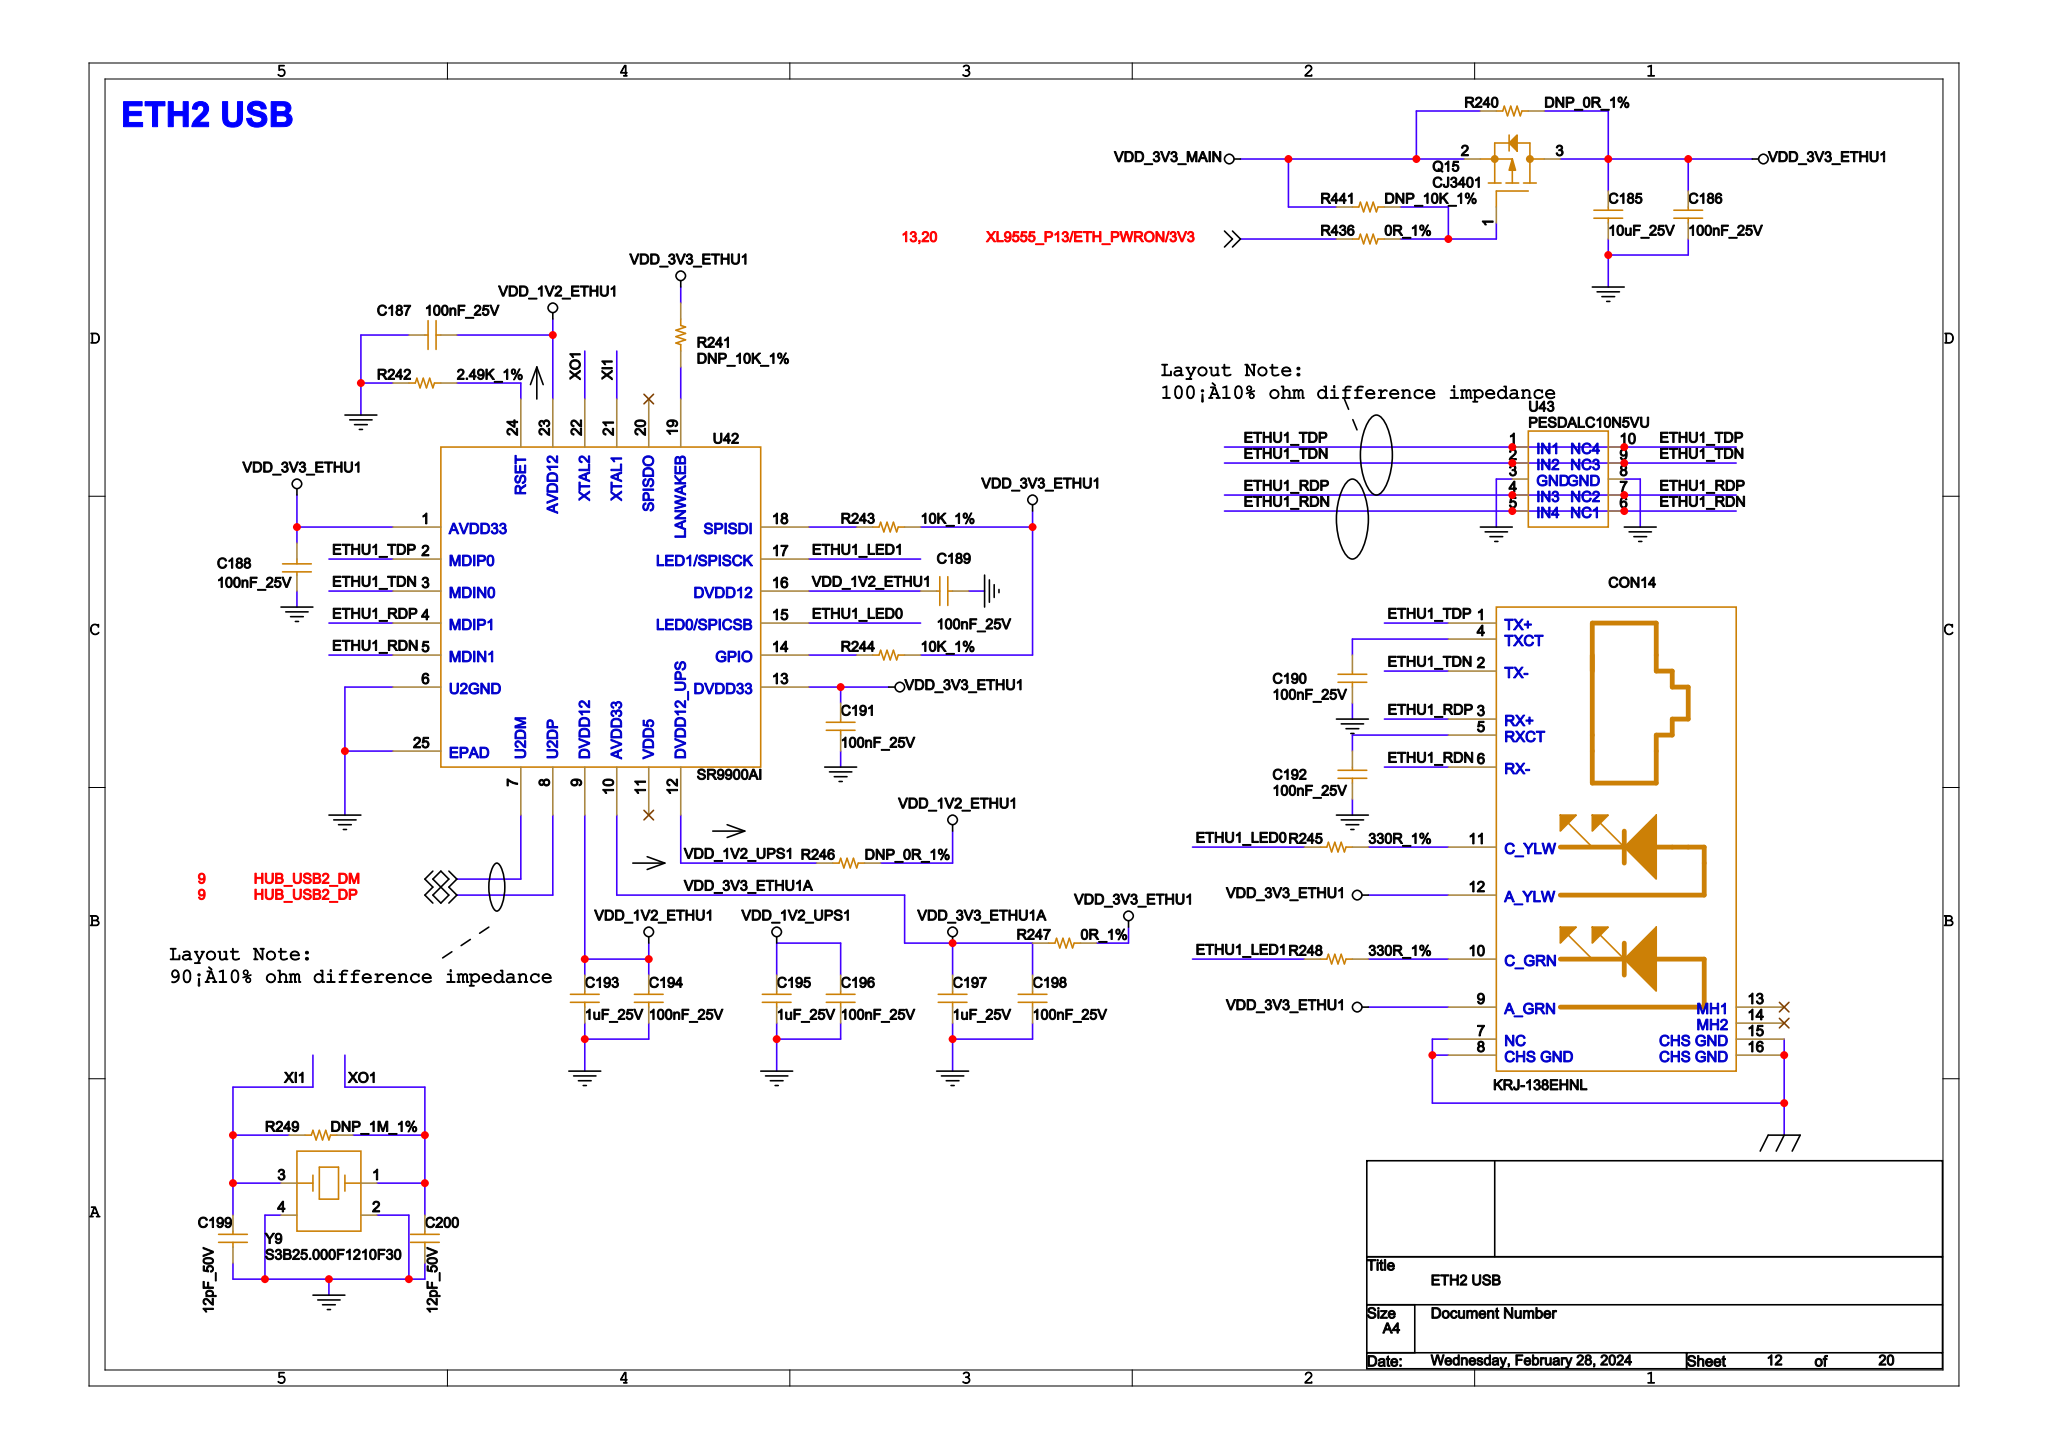Circuit board | Cadence Allegro | 1024 parts | 682 nets | one sheet of the schematic
Parts on this sheet (reference | value | footprint):
C185 | 10uF_25V | C0603
C186 | 100nF_25V | C0402
C187 | 100nF_25V | C0402
C188 | 100nF_25V | C0402
C189 | 100nF_25V | C0402
C190 | 100nF_25V | C0402
C191 | 100nF_25V | C0402
C192 | 100nF_25V | C0402
C193 | 1uF_25V | C0603
C194 | 100nF_25V | C0402
C195 | 1uF_25V | C0603
C196 | 100nF_25V | C0402
C197 | 1uF_25V | C0603
C198 | 100nF_25V | C0402
C199 | 12pF_50V | C0402
C200 | 12pF_50V | C0402
CON14 | KRJ-138EHNL | CON_YDS_13F-64GYD2PLXNL
Q15 | CJ3401 | SOT23-3
R240 | DNP_0R_1% | R0603
R241 | DNP_10K_1% | R0402
R242 | 2.49K_1% | R0603
R243 | 10K_1% | R0402
R244 | 10K_1% | R0402
R245 | 330R_1% | R0402
R246 | DNP_0R_1% | R0603
R247 | 0R_1% | R0603
R248 | 330R_1% | R0402
R249 | DNP_1M_1% | R0603
R436 | 0R_1% | R0402
R441 | DNP_10K_1% | R0402
U42 | SR9900AI | QFN24-4X4-0D5
U43 | PESDALC10N5VU | DFN-10-2510
Y9 | S3B25.000F1210F30 | SMD_3225
Nets of these parts (net: part-pin ...):
GND: C185-2 C186-2 C187-1 C188-1 C189-2 C190-2 C191-2 C192-2 C193-2 C194-2 C195-2 C196-2 C197-2 C198-2 C199-2 C200-2 R242-1 U43-3 U43-8 Y9-2 Y9-4 U42-6 U42-25
EGND: CON14-7 CON14-8 CON14-15 CON14-16
VDD_3V3_MAIN: Q15-2 R240-1 R441-1
XI1: C199-1 R249-2 Y9-3 U42-21
XO1: C200-1 R249-1 Y9-1 U42-22
VDD_3V3_ETHU1: C185-1 C186-1 C188-2 C191-1 CON14-9 CON14-12 Q15-3 R240-2 R241-2 R243-2 R244-2 R247-2 U42-1 U42-13
N21671622: CON14-10 R248-2
N21671710: CON14-11 R245-2
ETHU1_RDP: CON14-3 U43-4 U43-7 U42-4
ETHU1_RDN: CON14-6 U43-5 U43-6 U42-5
N21671084: C192-1 CON14-5
ETHU1_TDP: CON14-1 U43-1 U43-10 U42-2
ETHU1_TDN: CON14-2 U43-2 U43-9 U42-3
N21671657: C190-1 CON14-4
VDD_1V2_UPS1: C195-1 C196-1 R246-1 U42-12
VDD_1V2_ETHU1: C187-2 C189-1 C193-1 C194-1 R246-2 U42-9 U42-16 U42-23
VDD_3V3_ETHU1A: C197-1 C198-1 R247-1 U42-10
N21671443: R242-2 U42-24
ETHU1_LED0: R245-1 U42-15
ETHU1_LED1: R248-1 U42-17
N21671469: R244-1 U42-14
N21671265: R241-1 U42-19
N21671454: R243-1 U42-18
HUB_USB2_DM: U42-7
HUB_USB2_DP: U42-8
XL9555_P13/ETH_PWRON/3V3: R436-2
N22258905: Q15-1 R436-1 R441-2